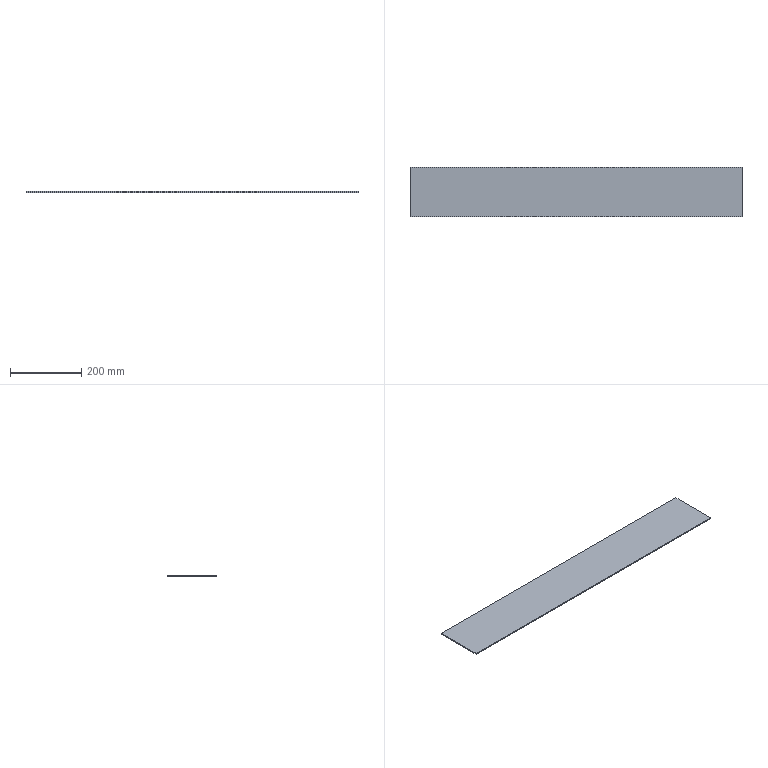Part | 1 solid | 6 faces | box 930 x 138 x 3 mm | volume 385020 mm3 | plane 6
STEP:
#1=CARTESIAN_POINT('',(-465.,69.,0.));
#2=VERTEX_POINT('',#1);
#3=CARTESIAN_POINT('',(-465.,-69.,0.));
#4=VERTEX_POINT('',#3);
#5=CARTESIAN_POINT('',(-465.,69.,0.));
#6=DIRECTION('',(0.,-1.,0.));
#7=VECTOR('',#6,1000.);
#8=LINE('',#5,#7);
#9=EDGE_CURVE('',#2,#4,#8,.T.);
#10=ORIENTED_EDGE('',*,*,#9,.T.);
#11=CARTESIAN_POINT('',(-465.,-69.,3.));
#12=VERTEX_POINT('',#11);
#13=CARTESIAN_POINT('',(-465.,-69.,3.));
#14=DIRECTION('',(0.,0.,-1.));
#15=VECTOR('',#14,1000.);
#16=LINE('',#13,#15);
#17=EDGE_CURVE('',#12,#4,#16,.T.);
#18=ORIENTED_EDGE('',*,*,#17,.F.);
#19=CARTESIAN_POINT('',(-465.,69.,3.));
#20=VERTEX_POINT('',#19);
#21=CARTESIAN_POINT('',(-465.,69.,3.));
#22=DIRECTION('',(0.,-1.,0.));
#23=VECTOR('',#22,1000.);
#24=LINE('',#21,#23);
#25=EDGE_CURVE('',#20,#12,#24,.T.);
#26=ORIENTED_EDGE('',*,*,#25,.F.);
#27=CARTESIAN_POINT('',(-465.,69.,3.));
#28=DIRECTION('',(0.,0.,-1.));
#29=VECTOR('',#28,1000.);
#30=LINE('',#27,#29);
#31=EDGE_CURVE('',#20,#2,#30,.T.);
#32=ORIENTED_EDGE('',*,*,#31,.T.);
#33=EDGE_LOOP('',(#10,#18,#26,#32));
#34=FACE_OUTER_BOUND('',#33,.T.);
#35=CARTESIAN_POINT('',(-465.,69.,3.));
#36=DIRECTION('',(1.,0.,0.));
#37=DIRECTION('',(0.,1.,0.));
#38=AXIS2_PLACEMENT_3D('',#35,#36,#37);
#39=PLANE('',#38);
#40=ADVANCED_FACE('',(#34),#39,.F.);
#41=CARTESIAN_POINT('',(465.,-69.,0.));
#42=VERTEX_POINT('',#41);
#43=CARTESIAN_POINT('',(-465.,-69.,0.));
#44=DIRECTION('',(1.,0.,0.));
#45=VECTOR('',#44,1000.);
#46=LINE('',#43,#45);
#47=EDGE_CURVE('',#4,#42,#46,.T.);
#48=ORIENTED_EDGE('',*,*,#47,.T.);
#49=CARTESIAN_POINT('',(465.,-69.,3.));
#50=VERTEX_POINT('',#49);
#51=CARTESIAN_POINT('',(465.,-69.,3.));
#52=DIRECTION('',(0.,0.,-1.));
#53=VECTOR('',#52,1000.);
#54=LINE('',#51,#53);
#55=EDGE_CURVE('',#50,#42,#54,.T.);
#56=ORIENTED_EDGE('',*,*,#55,.F.);
#57=CARTESIAN_POINT('',(-465.,-69.,3.));
#58=DIRECTION('',(1.,0.,0.));
#59=VECTOR('',#58,1000.);
#60=LINE('',#57,#59);
#61=EDGE_CURVE('',#12,#50,#60,.T.);
#62=ORIENTED_EDGE('',*,*,#61,.F.);
#63=ORIENTED_EDGE('',*,*,#17,.T.);
#64=EDGE_LOOP('',(#48,#56,#62,#63));
#65=FACE_OUTER_BOUND('',#64,.T.);
#66=CARTESIAN_POINT('',(-465.,-69.,3.));
#67=DIRECTION('',(0.,1.,0.));
#68=DIRECTION('',(1.,0.,0.));
#69=AXIS2_PLACEMENT_3D('',#66,#67,#68);
#70=PLANE('',#69);
#71=ADVANCED_FACE('',(#65),#70,.F.);
#72=CARTESIAN_POINT('',(465.,69.,0.));
#73=VERTEX_POINT('',#72);
#74=CARTESIAN_POINT('',(465.,69.,0.));
#75=DIRECTION('',(0.,-1.,0.));
#76=VECTOR('',#75,1000.);
#77=LINE('',#74,#76);
#78=EDGE_CURVE('',#73,#42,#77,.T.);
#79=ORIENTED_EDGE('',*,*,#78,.F.);
#80=CARTESIAN_POINT('',(465.,69.,3.));
#81=VERTEX_POINT('',#80);
#82=CARTESIAN_POINT('',(465.,69.,3.));
#83=DIRECTION('',(0.,0.,-1.));
#84=VECTOR('',#83,1000.);
#85=LINE('',#82,#84);
#86=EDGE_CURVE('',#81,#73,#85,.T.);
#87=ORIENTED_EDGE('',*,*,#86,.F.);
#88=CARTESIAN_POINT('',(465.,69.,3.));
#89=DIRECTION('',(0.,-1.,0.));
#90=VECTOR('',#89,1000.);
#91=LINE('',#88,#90);
#92=EDGE_CURVE('',#81,#50,#91,.T.);
#93=ORIENTED_EDGE('',*,*,#92,.T.);
#94=ORIENTED_EDGE('',*,*,#55,.T.);
#95=EDGE_LOOP('',(#79,#87,#93,#94));
#96=FACE_OUTER_BOUND('',#95,.T.);
#97=CARTESIAN_POINT('',(465.,69.,3.));
#98=DIRECTION('',(1.,0.,0.));
#99=DIRECTION('',(0.,1.,0.));
#100=AXIS2_PLACEMENT_3D('',#97,#98,#99);
#101=PLANE('',#100);
#102=ADVANCED_FACE('',(#96),#101,.T.);
#103=CARTESIAN_POINT('',(-465.,69.,0.));
#104=DIRECTION('',(1.,0.,0.));
#105=VECTOR('',#104,1000.);
#106=LINE('',#103,#105);
#107=EDGE_CURVE('',#2,#73,#106,.T.);
#108=ORIENTED_EDGE('',*,*,#107,.F.);
#109=ORIENTED_EDGE('',*,*,#31,.F.);
#110=CARTESIAN_POINT('',(-465.,69.,3.));
#111=DIRECTION('',(1.,0.,0.));
#112=VECTOR('',#111,1000.);
#113=LINE('',#110,#112);
#114=EDGE_CURVE('',#20,#81,#113,.T.);
#115=ORIENTED_EDGE('',*,*,#114,.T.);
#116=ORIENTED_EDGE('',*,*,#86,.T.);
#117=EDGE_LOOP('',(#108,#109,#115,#116));
#118=FACE_OUTER_BOUND('',#117,.T.);
#119=CARTESIAN_POINT('',(-465.,69.,3.));
#120=DIRECTION('',(0.,1.,0.));
#121=DIRECTION('',(1.,0.,0.));
#122=AXIS2_PLACEMENT_3D('',#119,#120,#121);
#123=PLANE('',#122);
#124=ADVANCED_FACE('',(#118),#123,.T.);
#125=ORIENTED_EDGE('',*,*,#25,.T.);
#126=ORIENTED_EDGE('',*,*,#61,.T.);
#127=ORIENTED_EDGE('',*,*,#92,.F.);
#128=ORIENTED_EDGE('',*,*,#114,.F.);
#129=EDGE_LOOP('',(#125,#126,#127,#128));
#130=FACE_OUTER_BOUND('',#129,.T.);
#131=CARTESIAN_POINT('',(0.,0.,3.));
#132=DIRECTION('',(0.,0.,1.));
#133=DIRECTION('',(1.,0.,0.));
#134=AXIS2_PLACEMENT_3D('',#131,#132,#133);
#135=PLANE('',#134);
#136=ADVANCED_FACE('',(#130),#135,.T.);
#137=ORIENTED_EDGE('',*,*,#9,.F.);
#138=ORIENTED_EDGE('',*,*,#107,.T.);
#139=ORIENTED_EDGE('',*,*,#78,.T.);
#140=ORIENTED_EDGE('',*,*,#47,.F.);
#141=EDGE_LOOP('',(#137,#138,#139,#140));
#142=FACE_OUTER_BOUND('',#141,.T.);
#143=CARTESIAN_POINT('',(0.,0.,0.));
#144=DIRECTION('',(0.,0.,1.));
#145=DIRECTION('',(1.,0.,0.));
#146=AXIS2_PLACEMENT_3D('',#143,#144,#145);
#147=PLANE('',#146);
#148=ADVANCED_FACE('',(#142),#147,.F.);
#149=CLOSED_SHELL('',(#40,#71,#102,#124,#136,#148));
#150=MANIFOLD_SOLID_BREP('',#149);
#151=CARTESIAN_POINT('',(0.,0.,0.));
#152=DIRECTION('',(0.,0.,1.));
#153=DIRECTION('',(1.,0.,0.));
#154=AXIS2_PLACEMENT_3D('',#151,#152,#153);
#155=(LENGTH_UNIT()NAMED_UNIT(*)SI_UNIT(.MILLI.,.METRE.));
#156=UNCERTAINTY_MEASURE_WITH_UNIT(LENGTH_MEASURE(0.00001),#155,'','');
#157=(NAMED_UNIT(*)PLANE_ANGLE_UNIT()SI_UNIT($,.RADIAN.));
#158=(NAMED_UNIT(*)SI_UNIT($,.STERADIAN.)SOLID_ANGLE_UNIT());
#159=(GEOMETRIC_REPRESENTATION_CONTEXT(3)GLOBAL_UNCERTAINTY_ASSIGNED_CONTEXT((#156))GLOBAL_UNIT_ASSIGNED_CONTEXT((#155,#157,#158))REPRESENTATION_CONTEXT('',''));
#160=ADVANCED_BREP_SHAPE_REPRESENTATION('',(#150,#154),#159);